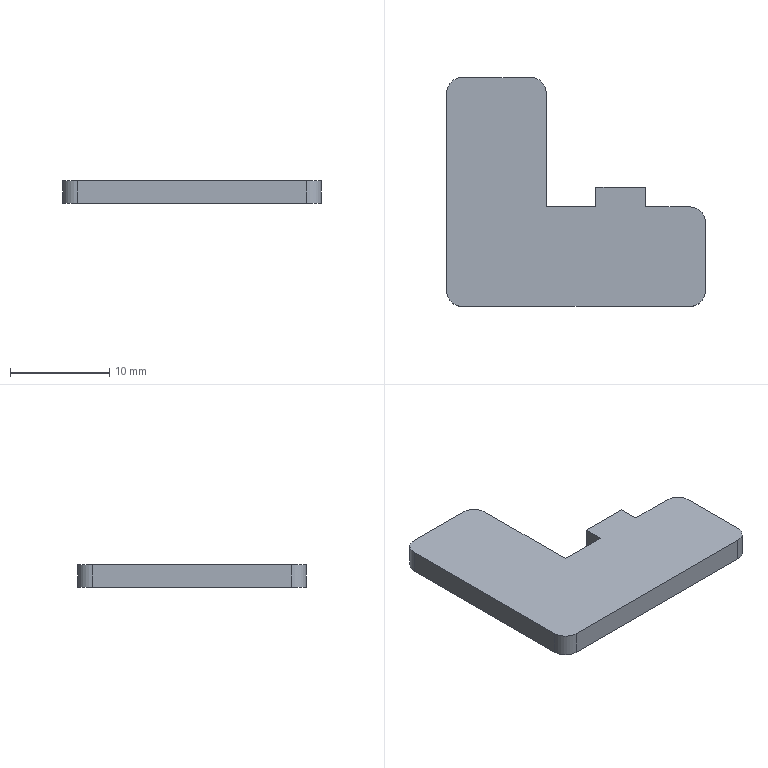Part | SolidWorks | features FlatPattern 1, SMBaseFlange 1, SheetMetal 1 | 1 solid | 17 faces | box 26 x 23 x 2.3 mm | volume 914.447 mm3 | plane 12 | cylinder 5 | commonest cylinder face diameters 3 x5
STEP:
#1=CARTESIAN_POINT('',(1215.997,-3.8,0.));
#2=VERTEX_POINT('',#1);
#3=CARTESIAN_POINT('',(1214.497,-2.3,0.));
#4=VERTEX_POINT('',#3);
#5=CARTESIAN_POINT('',(1214.497,-3.8,0.));
#6=DIRECTION('',(0.,0.,1.));
#7=DIRECTION('',(1.,0.,0.));
#8=AXIS2_PLACEMENT_3D('',#5,#6,#7);
#9=CIRCLE('',#8,1.5);
#10=EDGE_CURVE('',#2,#4,#9,.T.);
#11=ORIENTED_EDGE('',*,*,#10,.T.);
#12=CARTESIAN_POINT('',(1214.497,-2.3,2.3));
#13=VERTEX_POINT('',#12);
#14=CARTESIAN_POINT('',(1214.497,-2.3,2.3));
#15=DIRECTION('',(0.,0.,-1.));
#16=VECTOR('',#15,1000.);
#17=LINE('',#14,#16);
#18=EDGE_CURVE('',#13,#4,#17,.T.);
#19=ORIENTED_EDGE('',*,*,#18,.F.);
#20=CARTESIAN_POINT('',(1215.997,-3.8,2.3));
#21=VERTEX_POINT('',#20);
#22=CARTESIAN_POINT('',(1214.497,-3.8,2.3));
#23=DIRECTION('',(0.,0.,1.));
#24=DIRECTION('',(1.,0.,0.));
#25=AXIS2_PLACEMENT_3D('',#22,#23,#24);
#26=CIRCLE('',#25,1.5);
#27=EDGE_CURVE('',#21,#13,#26,.T.);
#28=ORIENTED_EDGE('',*,*,#27,.F.);
#29=CARTESIAN_POINT('',(1215.997,-3.8,2.3));
#30=DIRECTION('',(0.,0.,-1.));
#31=VECTOR('',#30,1000.);
#32=LINE('',#29,#31);
#33=EDGE_CURVE('',#21,#2,#32,.T.);
#34=ORIENTED_EDGE('',*,*,#33,.T.);
#35=EDGE_LOOP('',(#11,#19,#28,#34));
#36=FACE_OUTER_BOUND('',#35,.T.);
#37=CARTESIAN_POINT('',(1214.497,-3.8,2.3));
#38=DIRECTION('',(0.,0.,-1.));
#39=DIRECTION('',(-1.,0.,0.));
#40=AXIS2_PLACEMENT_3D('',#37,#38,#39);
#41=CYLINDRICAL_SURFACE('',#40,1.5);
#42=ADVANCED_FACE('',(#36),#41,.T.);
#43=CARTESIAN_POINT('',(1209.997,-2.3,0.));
#44=VERTEX_POINT('',#43);
#45=CARTESIAN_POINT('',(1209.997,-2.3,0.));
#46=DIRECTION('',(-1.,0.,0.));
#47=VECTOR('',#46,1000.);
#48=LINE('',#45,#47);
#49=EDGE_CURVE('',#4,#44,#48,.T.);
#50=ORIENTED_EDGE('',*,*,#49,.T.);
#51=CARTESIAN_POINT('',(1209.997,-2.3,2.3));
#52=VERTEX_POINT('',#51);
#53=CARTESIAN_POINT('',(1209.997,-2.3,2.3));
#54=DIRECTION('',(0.,0.,-1.));
#55=VECTOR('',#54,1000.);
#56=LINE('',#53,#55);
#57=EDGE_CURVE('',#52,#44,#56,.T.);
#58=ORIENTED_EDGE('',*,*,#57,.F.);
#59=CARTESIAN_POINT('',(1209.997,-2.3,2.3));
#60=DIRECTION('',(-1.,0.,0.));
#61=VECTOR('',#60,1000.);
#62=LINE('',#59,#61);
#63=EDGE_CURVE('',#13,#52,#62,.T.);
#64=ORIENTED_EDGE('',*,*,#63,.F.);
#65=ORIENTED_EDGE('',*,*,#18,.T.);
#66=EDGE_LOOP('',(#50,#58,#64,#65));
#67=FACE_OUTER_BOUND('',#66,.T.);
#68=CARTESIAN_POINT('',(1209.997,-2.3,2.3));
#69=DIRECTION('',(0.,-1.,0.));
#70=DIRECTION('',(1.,0.,0.));
#71=AXIS2_PLACEMENT_3D('',#68,#69,#70);
#72=PLANE('',#71);
#73=ADVANCED_FACE('',(#67),#72,.F.);
#74=CARTESIAN_POINT('',(1209.997,-0.3,0.));
#75=VERTEX_POINT('',#74);
#76=CARTESIAN_POINT('',(1209.997,-0.3,0.));
#77=DIRECTION('',(0.,1.,0.));
#78=VECTOR('',#77,1000.);
#79=LINE('',#76,#78);
#80=EDGE_CURVE('',#44,#75,#79,.T.);
#81=ORIENTED_EDGE('',*,*,#80,.T.);
#82=CARTESIAN_POINT('',(1209.997,-0.3,2.3));
#83=VERTEX_POINT('',#82);
#84=CARTESIAN_POINT('',(1209.997,-0.3,2.3));
#85=DIRECTION('',(0.,0.,-1.));
#86=VECTOR('',#85,1000.);
#87=LINE('',#84,#86);
#88=EDGE_CURVE('',#83,#75,#87,.T.);
#89=ORIENTED_EDGE('',*,*,#88,.F.);
#90=CARTESIAN_POINT('',(1209.997,-0.3,2.3));
#91=DIRECTION('',(0.,1.,0.));
#92=VECTOR('',#91,1000.);
#93=LINE('',#90,#92);
#94=EDGE_CURVE('',#52,#83,#93,.T.);
#95=ORIENTED_EDGE('',*,*,#94,.F.);
#96=ORIENTED_EDGE('',*,*,#57,.T.);
#97=EDGE_LOOP('',(#81,#89,#95,#96));
#98=FACE_OUTER_BOUND('',#97,.T.);
#99=CARTESIAN_POINT('',(1209.997,-0.3,2.3));
#100=DIRECTION('',(-1.,0.,0.));
#101=DIRECTION('',(0.,0.,1.));
#102=AXIS2_PLACEMENT_3D('',#99,#100,#101);
#103=PLANE('',#102);
#104=ADVANCED_FACE('',(#98),#103,.F.);
#105=CARTESIAN_POINT('',(1204.997,-0.3,0.));
#106=VERTEX_POINT('',#105);
#107=CARTESIAN_POINT('',(1204.997,-0.3,0.));
#108=DIRECTION('',(-1.,0.,0.));
#109=VECTOR('',#108,1000.);
#110=LINE('',#107,#109);
#111=EDGE_CURVE('',#75,#106,#110,.T.);
#112=ORIENTED_EDGE('',*,*,#111,.T.);
#113=CARTESIAN_POINT('',(1204.997,-0.3,2.3));
#114=VERTEX_POINT('',#113);
#115=CARTESIAN_POINT('',(1204.997,-0.3,2.3));
#116=DIRECTION('',(0.,0.,-1.));
#117=VECTOR('',#116,1000.);
#118=LINE('',#115,#117);
#119=EDGE_CURVE('',#114,#106,#118,.T.);
#120=ORIENTED_EDGE('',*,*,#119,.F.);
#121=CARTESIAN_POINT('',(1204.997,-0.3,2.3));
#122=DIRECTION('',(-1.,0.,0.));
#123=VECTOR('',#122,1000.);
#124=LINE('',#121,#123);
#125=EDGE_CURVE('',#83,#114,#124,.T.);
#126=ORIENTED_EDGE('',*,*,#125,.F.);
#127=ORIENTED_EDGE('',*,*,#88,.T.);
#128=EDGE_LOOP('',(#112,#120,#126,#127));
#129=FACE_OUTER_BOUND('',#128,.T.);
#130=CARTESIAN_POINT('',(1204.997,-0.3,2.3));
#131=DIRECTION('',(0.,-1.,0.));
#132=DIRECTION('',(0.,0.,-1.));
#133=AXIS2_PLACEMENT_3D('',#130,#131,#132);
#134=PLANE('',#133);
#135=ADVANCED_FACE('',(#129),#134,.F.);
#136=CARTESIAN_POINT('',(1204.997,-2.3,0.));
#137=VERTEX_POINT('',#136);
#138=CARTESIAN_POINT('',(1204.997,-2.3,0.));
#139=DIRECTION('',(0.,-1.,0.));
#140=VECTOR('',#139,1000.);
#141=LINE('',#138,#140);
#142=EDGE_CURVE('',#106,#137,#141,.T.);
#143=ORIENTED_EDGE('',*,*,#142,.T.);
#144=CARTESIAN_POINT('',(1204.997,-2.3,2.3));
#145=VERTEX_POINT('',#144);
#146=CARTESIAN_POINT('',(1204.997,-2.3,2.3));
#147=DIRECTION('',(0.,0.,-1.));
#148=VECTOR('',#147,1000.);
#149=LINE('',#146,#148);
#150=EDGE_CURVE('',#145,#137,#149,.T.);
#151=ORIENTED_EDGE('',*,*,#150,.F.);
#152=CARTESIAN_POINT('',(1204.997,-2.3,2.3));
#153=DIRECTION('',(0.,-1.,0.));
#154=VECTOR('',#153,1000.);
#155=LINE('',#152,#154);
#156=EDGE_CURVE('',#114,#145,#155,.T.);
#157=ORIENTED_EDGE('',*,*,#156,.F.);
#158=ORIENTED_EDGE('',*,*,#119,.T.);
#159=EDGE_LOOP('',(#143,#151,#157,#158));
#160=FACE_OUTER_BOUND('',#159,.T.);
#161=CARTESIAN_POINT('',(1204.997,-2.3,2.3));
#162=DIRECTION('',(1.,0.,0.));
#163=DIRECTION('',(0.,1.,0.));
#164=AXIS2_PLACEMENT_3D('',#161,#162,#163);
#165=PLANE('',#164);
#166=ADVANCED_FACE('',(#160),#165,.F.);
#167=CARTESIAN_POINT('',(1199.997,-2.3,0.));
#168=VERTEX_POINT('',#167);
#169=CARTESIAN_POINT('',(1199.997,-2.3,0.));
#170=DIRECTION('',(-1.,0.,0.));
#171=VECTOR('',#170,1000.);
#172=LINE('',#169,#171);
#173=EDGE_CURVE('',#137,#168,#172,.T.);
#174=ORIENTED_EDGE('',*,*,#173,.T.);
#175=CARTESIAN_POINT('',(1199.997,-2.3,2.3));
#176=VERTEX_POINT('',#175);
#177=CARTESIAN_POINT('',(1199.997,-2.3,2.3));
#178=DIRECTION('',(0.,0.,-1.));
#179=VECTOR('',#178,1000.);
#180=LINE('',#177,#179);
#181=EDGE_CURVE('',#176,#168,#180,.T.);
#182=ORIENTED_EDGE('',*,*,#181,.F.);
#183=CARTESIAN_POINT('',(1199.997,-2.3,2.3));
#184=DIRECTION('',(-1.,0.,0.));
#185=VECTOR('',#184,1000.);
#186=LINE('',#183,#185);
#187=EDGE_CURVE('',#145,#176,#186,.T.);
#188=ORIENTED_EDGE('',*,*,#187,.F.);
#189=ORIENTED_EDGE('',*,*,#150,.T.);
#190=EDGE_LOOP('',(#174,#182,#188,#189));
#191=FACE_OUTER_BOUND('',#190,.T.);
#192=CARTESIAN_POINT('',(1199.997,-2.3,2.3));
#193=DIRECTION('',(0.,-1.,0.));
#194=DIRECTION('',(0.,0.,-1.));
#195=AXIS2_PLACEMENT_3D('',#192,#193,#194);
#196=PLANE('',#195);
#197=ADVANCED_FACE('',(#191),#196,.F.);
#198=CARTESIAN_POINT('',(1199.997,9.2,0.));
#199=VERTEX_POINT('',#198);
#200=CARTESIAN_POINT('',(1199.997,-2.3,0.));
#201=DIRECTION('',(0.,1.,0.));
#202=VECTOR('',#201,1000.);
#203=LINE('',#200,#202);
#204=EDGE_CURVE('',#168,#199,#203,.T.);
#205=ORIENTED_EDGE('',*,*,#204,.T.);
#206=CARTESIAN_POINT('',(1199.997,9.2,2.3));
#207=VERTEX_POINT('',#206);
#208=CARTESIAN_POINT('',(1199.997,9.2,2.3));
#209=DIRECTION('',(0.,0.,-1.));
#210=VECTOR('',#209,1000.);
#211=LINE('',#208,#210);
#212=EDGE_CURVE('',#207,#199,#211,.T.);
#213=ORIENTED_EDGE('',*,*,#212,.F.);
#214=CARTESIAN_POINT('',(1199.997,-2.3,2.3));
#215=DIRECTION('',(0.,1.,0.));
#216=VECTOR('',#215,1000.);
#217=LINE('',#214,#216);
#218=EDGE_CURVE('',#176,#207,#217,.T.);
#219=ORIENTED_EDGE('',*,*,#218,.F.);
#220=ORIENTED_EDGE('',*,*,#181,.T.);
#221=EDGE_LOOP('',(#205,#213,#219,#220));
#222=FACE_OUTER_BOUND('',#221,.T.);
#223=CARTESIAN_POINT('',(1199.997,-2.3,2.3));
#224=DIRECTION('',(-1.,0.,0.));
#225=DIRECTION('',(0.,0.,1.));
#226=AXIS2_PLACEMENT_3D('',#223,#224,#225);
#227=PLANE('',#226);
#228=ADVANCED_FACE('',(#222),#227,.F.);
#229=CARTESIAN_POINT('',(1198.497,10.7,0.));
#230=VERTEX_POINT('',#229);
#231=CARTESIAN_POINT('',(1198.497,9.2,0.));
#232=DIRECTION('',(0.,0.,1.));
#233=DIRECTION('',(1.,0.,0.));
#234=AXIS2_PLACEMENT_3D('',#231,#232,#233);
#235=CIRCLE('',#234,1.5);
#236=EDGE_CURVE('',#199,#230,#235,.T.);
#237=ORIENTED_EDGE('',*,*,#236,.T.);
#238=CARTESIAN_POINT('',(1198.497,10.7,2.3));
#239=VERTEX_POINT('',#238);
#240=CARTESIAN_POINT('',(1198.497,10.7,2.3));
#241=DIRECTION('',(0.,0.,-1.));
#242=VECTOR('',#241,1000.);
#243=LINE('',#240,#242);
#244=EDGE_CURVE('',#239,#230,#243,.T.);
#245=ORIENTED_EDGE('',*,*,#244,.F.);
#246=CARTESIAN_POINT('',(1198.497,9.2,2.3));
#247=DIRECTION('',(0.,0.,1.));
#248=DIRECTION('',(1.,0.,0.));
#249=AXIS2_PLACEMENT_3D('',#246,#247,#248);
#250=CIRCLE('',#249,1.5);
#251=EDGE_CURVE('',#207,#239,#250,.T.);
#252=ORIENTED_EDGE('',*,*,#251,.F.);
#253=ORIENTED_EDGE('',*,*,#212,.T.);
#254=EDGE_LOOP('',(#237,#245,#252,#253));
#255=FACE_OUTER_BOUND('',#254,.T.);
#256=CARTESIAN_POINT('',(1198.497,9.2,2.3));
#257=DIRECTION('',(0.,0.,-1.));
#258=DIRECTION('',(-1.,0.,0.));
#259=AXIS2_PLACEMENT_3D('',#256,#257,#258);
#260=CYLINDRICAL_SURFACE('',#259,1.5);
#261=ADVANCED_FACE('',(#255),#260,.T.);
#262=CARTESIAN_POINT('',(1191.497,10.7,0.));
#263=VERTEX_POINT('',#262);
#264=CARTESIAN_POINT('',(1191.497,10.7,0.));
#265=DIRECTION('',(-1.,0.,0.));
#266=VECTOR('',#265,1000.);
#267=LINE('',#264,#266);
#268=EDGE_CURVE('',#230,#263,#267,.T.);
#269=ORIENTED_EDGE('',*,*,#268,.T.);
#270=CARTESIAN_POINT('',(1191.497,10.7,2.3));
#271=VERTEX_POINT('',#270);
#272=CARTESIAN_POINT('',(1191.497,10.7,2.3));
#273=DIRECTION('',(0.,0.,-1.));
#274=VECTOR('',#273,1000.);
#275=LINE('',#272,#274);
#276=EDGE_CURVE('',#271,#263,#275,.T.);
#277=ORIENTED_EDGE('',*,*,#276,.F.);
#278=CARTESIAN_POINT('',(1191.497,10.7,2.3));
#279=DIRECTION('',(-1.,0.,0.));
#280=VECTOR('',#279,1000.);
#281=LINE('',#278,#280);
#282=EDGE_CURVE('',#239,#271,#281,.T.);
#283=ORIENTED_EDGE('',*,*,#282,.F.);
#284=ORIENTED_EDGE('',*,*,#244,.T.);
#285=EDGE_LOOP('',(#269,#277,#283,#284));
#286=FACE_OUTER_BOUND('',#285,.T.);
#287=CARTESIAN_POINT('',(1191.497,10.7,2.3));
#288=DIRECTION('',(0.,-1.,0.));
#289=DIRECTION('',(1.,0.,0.));
#290=AXIS2_PLACEMENT_3D('',#287,#288,#289);
#291=PLANE('',#290);
#292=ADVANCED_FACE('',(#286),#291,.F.);
#293=CARTESIAN_POINT('',(1189.997,9.2,0.));
#294=VERTEX_POINT('',#293);
#295=CARTESIAN_POINT('',(1191.497,9.2,0.));
#296=DIRECTION('',(0.,0.,1.));
#297=DIRECTION('',(-1.,0.,0.));
#298=AXIS2_PLACEMENT_3D('',#295,#296,#297);
#299=CIRCLE('',#298,1.5);
#300=EDGE_CURVE('',#263,#294,#299,.T.);
#301=ORIENTED_EDGE('',*,*,#300,.T.);
#302=CARTESIAN_POINT('',(1189.997,9.2,2.3));
#303=VERTEX_POINT('',#302);
#304=CARTESIAN_POINT('',(1189.997,9.2,2.3));
#305=DIRECTION('',(0.,0.,-1.));
#306=VECTOR('',#305,1000.);
#307=LINE('',#304,#306);
#308=EDGE_CURVE('',#303,#294,#307,.T.);
#309=ORIENTED_EDGE('',*,*,#308,.F.);
#310=CARTESIAN_POINT('',(1191.497,9.2,2.3));
#311=DIRECTION('',(0.,0.,1.));
#312=DIRECTION('',(-1.,0.,0.));
#313=AXIS2_PLACEMENT_3D('',#310,#311,#312);
#314=CIRCLE('',#313,1.5);
#315=EDGE_CURVE('',#271,#303,#314,.T.);
#316=ORIENTED_EDGE('',*,*,#315,.F.);
#317=ORIENTED_EDGE('',*,*,#276,.T.);
#318=EDGE_LOOP('',(#301,#309,#316,#317));
#319=FACE_OUTER_BOUND('',#318,.T.);
#320=CARTESIAN_POINT('',(1191.497,9.2,2.3));
#321=DIRECTION('',(0.,0.,-1.));
#322=DIRECTION('',(-1.,0.,0.));
#323=AXIS2_PLACEMENT_3D('',#320,#321,#322);
#324=CYLINDRICAL_SURFACE('',#323,1.5);
#325=ADVANCED_FACE('',(#319),#324,.T.);
#326=CARTESIAN_POINT('',(1189.997,-10.8,0.));
#327=VERTEX_POINT('',#326);
#328=CARTESIAN_POINT('',(1189.997,-10.8,0.));
#329=DIRECTION('',(0.,-1.,0.));
#330=VECTOR('',#329,1000.);
#331=LINE('',#328,#330);
#332=EDGE_CURVE('',#294,#327,#331,.T.);
#333=ORIENTED_EDGE('',*,*,#332,.T.);
#334=CARTESIAN_POINT('',(1189.997,-10.8,2.3));
#335=VERTEX_POINT('',#334);
#336=CARTESIAN_POINT('',(1189.997,-10.8,2.3));
#337=DIRECTION('',(0.,0.,-1.));
#338=VECTOR('',#337,1000.);
#339=LINE('',#336,#338);
#340=EDGE_CURVE('',#335,#327,#339,.T.);
#341=ORIENTED_EDGE('',*,*,#340,.F.);
#342=CARTESIAN_POINT('',(1189.997,-10.8,2.3));
#343=DIRECTION('',(0.,-1.,0.));
#344=VECTOR('',#343,1000.);
#345=LINE('',#342,#344);
#346=EDGE_CURVE('',#303,#335,#345,.T.);
#347=ORIENTED_EDGE('',*,*,#346,.F.);
#348=ORIENTED_EDGE('',*,*,#308,.T.);
#349=EDGE_LOOP('',(#333,#341,#347,#348));
#350=FACE_OUTER_BOUND('',#349,.T.);
#351=CARTESIAN_POINT('',(1189.997,-10.8,2.3));
#352=DIRECTION('',(1.,0.,0.));
#353=DIRECTION('',(0.,0.,-1.));
#354=AXIS2_PLACEMENT_3D('',#351,#352,#353);
#355=PLANE('',#354);
#356=ADVANCED_FACE('',(#350),#355,.F.);
#357=CARTESIAN_POINT('',(1191.497,-12.3,0.));
#358=VERTEX_POINT('',#357);
#359=CARTESIAN_POINT('',(1191.497,-10.8,0.));
#360=DIRECTION('',(0.,0.,1.));
#361=DIRECTION('',(-1.,0.,0.));
#362=AXIS2_PLACEMENT_3D('',#359,#360,#361);
#363=CIRCLE('',#362,1.5);
#364=EDGE_CURVE('',#327,#358,#363,.T.);
#365=ORIENTED_EDGE('',*,*,#364,.T.);
#366=CARTESIAN_POINT('',(1191.497,-12.3,2.3));
#367=VERTEX_POINT('',#366);
#368=CARTESIAN_POINT('',(1191.497,-12.3,2.3));
#369=DIRECTION('',(0.,0.,-1.));
#370=VECTOR('',#369,1000.);
#371=LINE('',#368,#370);
#372=EDGE_CURVE('',#367,#358,#371,.T.);
#373=ORIENTED_EDGE('',*,*,#372,.F.);
#374=CARTESIAN_POINT('',(1191.497,-10.8,2.3));
#375=DIRECTION('',(0.,0.,1.));
#376=DIRECTION('',(-1.,0.,0.));
#377=AXIS2_PLACEMENT_3D('',#374,#375,#376);
#378=CIRCLE('',#377,1.5);
#379=EDGE_CURVE('',#335,#367,#378,.T.);
#380=ORIENTED_EDGE('',*,*,#379,.F.);
#381=ORIENTED_EDGE('',*,*,#340,.T.);
#382=EDGE_LOOP('',(#365,#373,#380,#381));
#383=FACE_OUTER_BOUND('',#382,.T.);
#384=CARTESIAN_POINT('',(1191.497,-10.8,2.3));
#385=DIRECTION('',(0.,0.,-1.));
#386=DIRECTION('',(-1.,0.,0.));
#387=AXIS2_PLACEMENT_3D('',#384,#385,#386);
#388=CYLINDRICAL_SURFACE('',#387,1.5);
#389=ADVANCED_FACE('',(#383),#388,.T.);
#390=CARTESIAN_POINT('',(1214.497,-12.3,0.));
#391=VERTEX_POINT('',#390);
#392=CARTESIAN_POINT('',(1214.497,-12.3,0.));
#393=DIRECTION('',(1.,0.,0.));
#394=VECTOR('',#393,1000.);
#395=LINE('',#392,#394);
#396=EDGE_CURVE('',#358,#391,#395,.T.);
#397=ORIENTED_EDGE('',*,*,#396,.T.);
#398=CARTESIAN_POINT('',(1214.497,-12.3,2.3));
#399=VERTEX_POINT('',#398);
#400=CARTESIAN_POINT('',(1214.497,-12.3,2.3));
#401=DIRECTION('',(0.,0.,-1.));
#402=VECTOR('',#401,1000.);
#403=LINE('',#400,#402);
#404=EDGE_CURVE('',#399,#391,#403,.T.);
#405=ORIENTED_EDGE('',*,*,#404,.F.);
#406=CARTESIAN_POINT('',(1214.497,-12.3,2.3));
#407=DIRECTION('',(1.,0.,0.));
#408=VECTOR('',#407,1000.);
#409=LINE('',#406,#408);
#410=EDGE_CURVE('',#367,#399,#409,.T.);
#411=ORIENTED_EDGE('',*,*,#410,.F.);
#412=ORIENTED_EDGE('',*,*,#372,.T.);
#413=EDGE_LOOP('',(#397,#405,#411,#412));
#414=FACE_OUTER_BOUND('',#413,.T.);
#415=CARTESIAN_POINT('',(1214.497,-12.3,2.3));
#416=DIRECTION('',(0.,1.,0.));
#417=DIRECTION('',(-1.,0.,0.));
#418=AXIS2_PLACEMENT_3D('',#415,#416,#417);
#419=PLANE('',#418);
#420=ADVANCED_FACE('',(#414),#419,.F.);
#421=CARTESIAN_POINT('',(1215.997,-10.8,0.));
#422=VERTEX_POINT('',#421);
#423=CARTESIAN_POINT('',(1214.497,-10.8,0.));
#424=DIRECTION('',(0.,0.,1.));
#425=DIRECTION('',(-1.,0.,0.));
#426=AXIS2_PLACEMENT_3D('',#423,#424,#425);
#427=CIRCLE('',#426,1.5);
#428=EDGE_CURVE('',#391,#422,#427,.T.);
#429=ORIENTED_EDGE('',*,*,#428,.T.);
#430=CARTESIAN_POINT('',(1215.997,-10.8,2.3));
#431=VERTEX_POINT('',#430);
#432=CARTESIAN_POINT('',(1215.997,-10.8,2.3));
#433=DIRECTION('',(0.,0.,-1.));
#434=VECTOR('',#433,1000.);
#435=LINE('',#432,#434);
#436=EDGE_CURVE('',#431,#422,#435,.T.);
#437=ORIENTED_EDGE('',*,*,#436,.F.);
#438=CARTESIAN_POINT('',(1214.497,-10.8,2.3));
#439=DIRECTION('',(0.,0.,1.));
#440=DIRECTION('',(-1.,0.,0.));
#441=AXIS2_PLACEMENT_3D('',#438,#439,#440);
#442=CIRCLE('',#441,1.5);
#443=EDGE_CURVE('',#399,#431,#442,.T.);
#444=ORIENTED_EDGE('',*,*,#443,.F.);
#445=ORIENTED_EDGE('',*,*,#404,.T.);
#446=EDGE_LOOP('',(#429,#437,#444,#445));
#447=FACE_OUTER_BOUND('',#446,.T.);
#448=CARTESIAN_POINT('',(1214.497,-10.8,2.3));
#449=DIRECTION('',(0.,0.,-1.));
#450=DIRECTION('',(-1.,0.,0.));
#451=AXIS2_PLACEMENT_3D('',#448,#449,#450);
#452=CYLINDRICAL_SURFACE('',#451,1.5);
#453=ADVANCED_FACE('',(#447),#452,.T.);
#454=CARTESIAN_POINT('',(1215.997,-3.8,0.));
#455=DIRECTION('',(0.,1.,0.));
#456=VECTOR('',#455,1000.);
#457=LINE('',#454,#456);
#458=EDGE_CURVE('',#422,#2,#457,.T.);
#459=ORIENTED_EDGE('',*,*,#458,.T.);
#460=ORIENTED_EDGE('',*,*,#33,.F.);
#461=CARTESIAN_POINT('',(1215.997,-3.8,2.3));
#462=DIRECTION('',(0.,1.,0.));
#463=VECTOR('',#462,1000.);
#464=LINE('',#461,#463);
#465=EDGE_CURVE('',#431,#21,#464,.T.);
#466=ORIENTED_EDGE('',*,*,#465,.F.);
#467=ORIENTED_EDGE('',*,*,#436,.T.);
#468=EDGE_LOOP('',(#459,#460,#466,#467));
#469=FACE_OUTER_BOUND('',#468,.T.);
#470=CARTESIAN_POINT('',(1215.997,-3.8,2.3));
#471=DIRECTION('',(-1.,0.,0.));
#472=DIRECTION('',(0.,0.,1.));
#473=AXIS2_PLACEMENT_3D('',#470,#471,#472);
#474=PLANE('',#473);
#475=ADVANCED_FACE('',(#469),#474,.F.);
#476=ORIENTED_EDGE('',*,*,#27,.T.);
#477=ORIENTED_EDGE('',*,*,#63,.T.);
#478=ORIENTED_EDGE('',*,*,#94,.T.);
#479=ORIENTED_EDGE('',*,*,#125,.T.);
#480=ORIENTED_EDGE('',*,*,#156,.T.);
#481=ORIENTED_EDGE('',*,*,#187,.T.);
#482=ORIENTED_EDGE('',*,*,#218,.T.);
#483=ORIENTED_EDGE('',*,*,#251,.T.);
#484=ORIENTED_EDGE('',*,*,#282,.T.);
#485=ORIENTED_EDGE('',*,*,#315,.T.);
#486=ORIENTED_EDGE('',*,*,#346,.T.);
#487=ORIENTED_EDGE('',*,*,#379,.T.);
#488=ORIENTED_EDGE('',*,*,#410,.T.);
#489=ORIENTED_EDGE('',*,*,#443,.T.);
#490=ORIENTED_EDGE('',*,*,#465,.T.);
#491=EDGE_LOOP('',(#476,#477,#478,#479,#480,#481,#482,#483,#484,#485,#486,#487,#488,#489,#490));
#492=FACE_OUTER_BOUND('',#491,.T.);
#493=CARTESIAN_POINT('',(1214.497,-3.8,2.3));
#494=DIRECTION('',(0.,0.,1.));
#495=DIRECTION('',(1.,0.,0.));
#496=AXIS2_PLACEMENT_3D('',#493,#494,#495);
#497=PLANE('',#496);
#498=ADVANCED_FACE('',(#492),#497,.T.);
#499=ORIENTED_EDGE('',*,*,#10,.F.);
#500=ORIENTED_EDGE('',*,*,#458,.F.);
#501=ORIENTED_EDGE('',*,*,#428,.F.);
#502=ORIENTED_EDGE('',*,*,#396,.F.);
#503=ORIENTED_EDGE('',*,*,#364,.F.);
#504=ORIENTED_EDGE('',*,*,#332,.F.);
#505=ORIENTED_EDGE('',*,*,#300,.F.);
#506=ORIENTED_EDGE('',*,*,#268,.F.);
#507=ORIENTED_EDGE('',*,*,#236,.F.);
#508=ORIENTED_EDGE('',*,*,#204,.F.);
#509=ORIENTED_EDGE('',*,*,#173,.F.);
#510=ORIENTED_EDGE('',*,*,#142,.F.);
#511=ORIENTED_EDGE('',*,*,#111,.F.);
#512=ORIENTED_EDGE('',*,*,#80,.F.);
#513=ORIENTED_EDGE('',*,*,#49,.F.);
#514=EDGE_LOOP('',(#499,#500,#501,#502,#503,#504,#505,#506,#507,#508,#509,#510,#511,#512,#513));
#515=FACE_OUTER_BOUND('',#514,.T.);
#516=CARTESIAN_POINT('',(1214.497,-3.8,0.));
#517=DIRECTION('',(0.,0.,1.));
#518=DIRECTION('',(1.,0.,0.));
#519=AXIS2_PLACEMENT_3D('',#516,#517,#518);
#520=PLANE('',#519);
#521=ADVANCED_FACE('',(#515),#520,.F.);
#522=CLOSED_SHELL('',(#42,#73,#104,#135,#166,#197,#228,#261,#292,#325,#356,#389,#420,#453,#475,#498,#521));
#523=MANIFOLD_SOLID_BREP('',#522);
#524=CARTESIAN_POINT('',(0.,0.,0.));
#525=DIRECTION('',(0.,0.,1.));
#526=DIRECTION('',(1.,0.,0.));
#527=AXIS2_PLACEMENT_3D('',#524,#525,#526);
#528=(LENGTH_UNIT()NAMED_UNIT(*)SI_UNIT(.MILLI.,.METRE.));
#529=UNCERTAINTY_MEASURE_WITH_UNIT(LENGTH_MEASURE(0.00001),#528,'','');
#530=(NAMED_UNIT(*)PLANE_ANGLE_UNIT()SI_UNIT($,.RADIAN.));
#531=(NAMED_UNIT(*)SI_UNIT($,.STERADIAN.)SOLID_ANGLE_UNIT());
#532=(GEOMETRIC_REPRESENTATION_CONTEXT(3)GLOBAL_UNCERTAINTY_ASSIGNED_CONTEXT((#529))GLOBAL_UNIT_ASSIGNED_CONTEXT((#528,#530,#531))REPRESENTATION_CONTEXT('',''));
#533=ADVANCED_BREP_SHAPE_REPRESENTATION('',(#523,#527),#532);